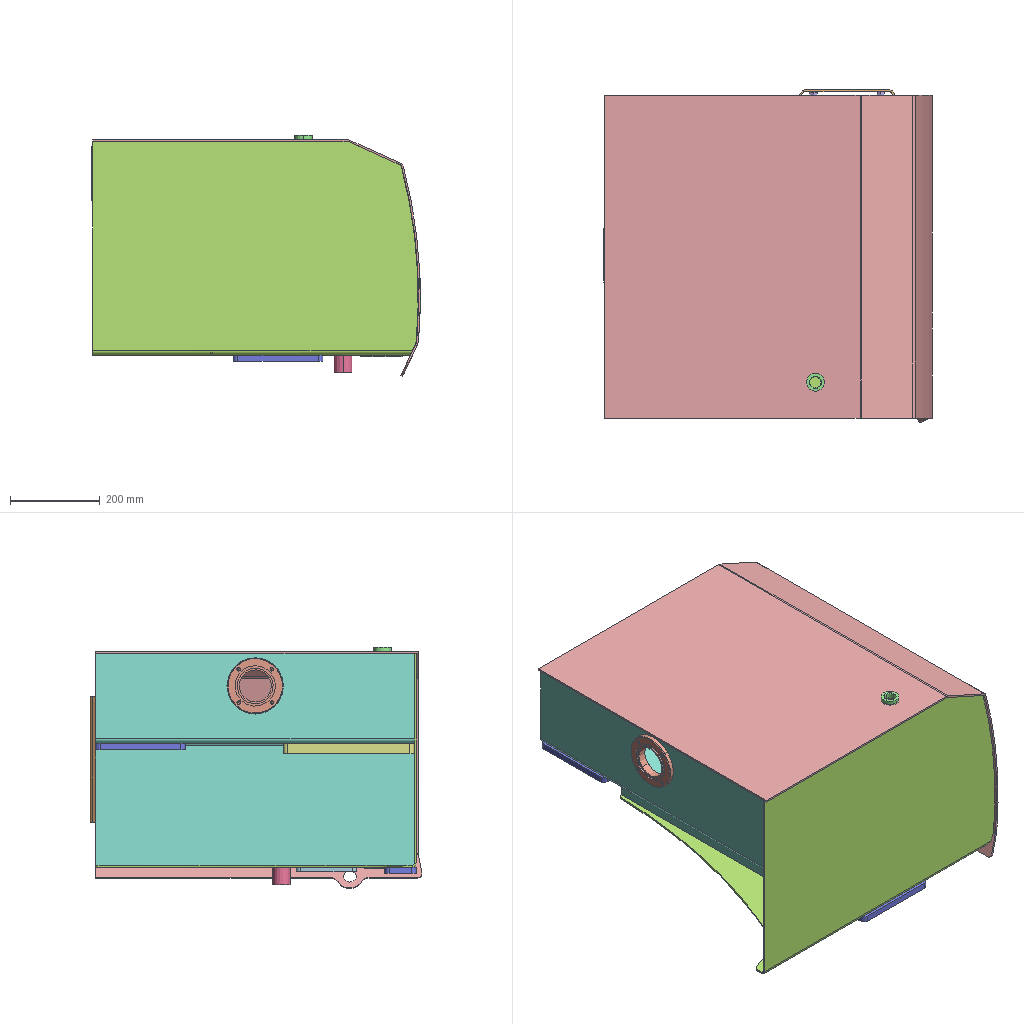Assembly | SolidWorks | 16 different items | 19 placed | box 733 x 740 x 538 mm
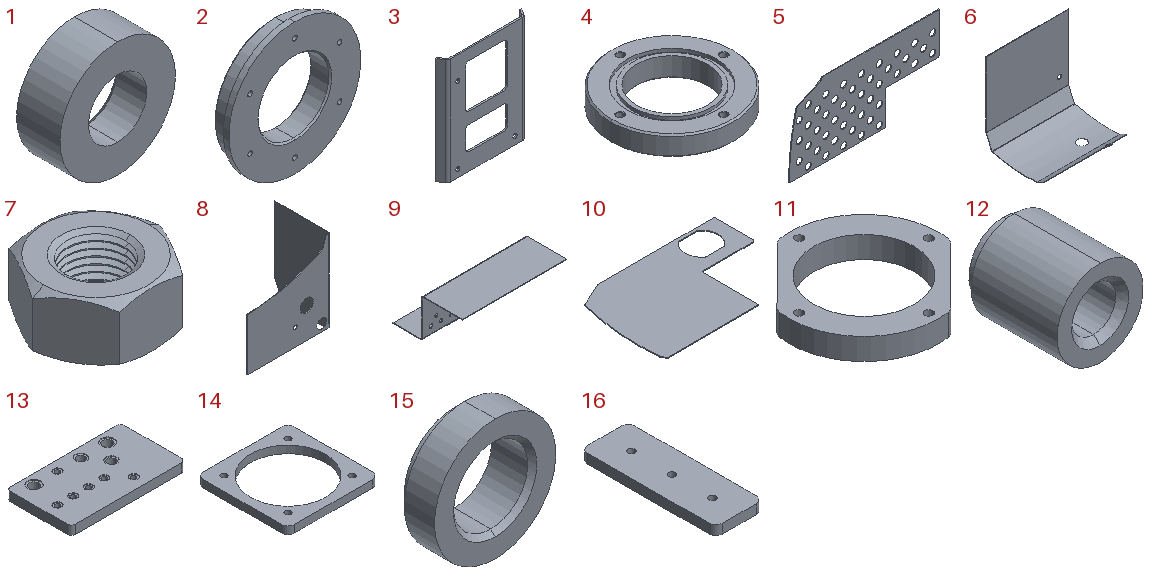Parts list (item | quantity | size | volume | features):
1 | x1 | 80 x 30 x 80 mm | 100918 mm3 | features HoleWzd 1, Revolution 1
2 | x1 | 93 x 14.5 x 93 mm | 57472 mm3 | features Chamfer 1, HoleWzd 1, Revolution 1
3 | x1 | 225 x 22.12 x 280 mm | 191805 mm3 | features FlatPattern 1, ICE 1, SMBaseFlange 1, SheetMetal 1
4 | x1 | 125 x 125 x 20 mm | 156275 mm3 | features Chamfer 2, ICE 2, FlatPattern 1, HoleWzd 1, SMBaseFlange 1, SheetMetal 1
5 | x1 | 714.557 x 4 x 360 mm | 695889 mm3 | features Extrusion 1
6 | x1 | 728.102 x 528.57 x 731.248 mm | 3316109 mm3 | features ICE 4, Fillet 1, FlatPattern 1, Fold 1, SMBaseFlange 1, SheetMetal 1, UnFold 1
7 | x3 | 18.475 x 16 x 8.4 mm | 1305 mm3 | features RevCut 2, Chamfer 1, Extrusion 1, LPattern 1
8 | x1 | 715 x 476 x 726.29 mm | 2754090 mm3 | features ICE 3, Fillet 2, FlatPattern 1, SMBaseFlange 1, SheetMetal 1
9 | x1 | 711 x 472 x 260 mm | 1991035 mm3 | features ICE 2, FlatPattern 1, SMBaseFlange 1, SheetMetal 1
10 | x1 | 714.283 x 472 x 4 mm | 956528 mm3 | features FlatPattern 1, SMBaseFlange 1, SheetMetal 1
11 | x1 | 158 x 158 x 23 mm | 204311 mm3 | features FlatPattern 1, HoleWzd 1, ICE 1, SMBaseFlange 1, SheetMetal 1
12 | x1 | 40 x 45 x 40 mm | 40970 mm3 | features Chamfer 1, Revolution 1
13 | x1 | 292 x 165 x 23 mm | 1047864 mm3 | features HoleWzd 4, ICE 3, FlatPattern 1, SMBaseFlange 1, SheetMetal 1
14 | x1 | 135 x 135 x 11 mm | 90588 mm3 | features FlatPattern 1, HoleWzd 1, SMBaseFlange 1, SheetMetal 1
15 | x1 | 40 x 13.5 x 40 mm | 9105 mm3 | features Chamfer 1, HoleWzd 1, Revolution 1
16 | x2 | 70 x 200 x 14 mm | 191366 mm3 | features FlatPattern 1, HoleWzd 1, SMBaseFlange 1, SheetMetal 1
Mates (type | each side: item.copy, entity, surface, feature):
Coincident | 6.1 face plane Base-Flange1 | 10.1 face plane Base-Flange1
DistanceDim | 6.1 face plane Base-Flange1 | 10.1 face plane Base-Flange1
DistanceDim | 10.1 face plane Base-Flange1 | 6.1 face plane Base-Flange1
Coincident | 6.1 face plane Base-Flange1 | 8.1 face plane Base-Flange1 | 2 times
DistanceDim | 8.1 face plane Base-Flange1 | 6.1 face plane Cut-Extrude2
Coincident | 6.1 face plane Base-Flange1 | 5.1 face plane Boss-Extrude1
DistanceDim | 6.1 face plane Base-Flange1 | 5.1 face plane Boss-Extrude1 | 2 times
Coincident | 10.1 face plane Base-Flange1 | 9.1 face plane Base-Flange1
Coincident | 6.1 face plane Base-Flange1 | 9.1 face plane Base-Flange1
Coincident | 8.1 face plane Base-Flange1 | 9.1 face plane Base-Flange1
DistanceDim | 10.1 face plane Base-Flange1 | 3.1 face plane Base-Flange1
DistanceDim | 9.1 face plane Base-Flange1 | 3.1 edge
DistanceDim | 8.1 face plane Base-Flange1 | 3.1 face plane Base-Flange1
Concentric | 3.1 face cylinder Cut-Extrude1 | 7.1 edge
Coincident | 3.1 face plane Base-Flange1 | 7.1 face plane BaseNut
Parallel | 7.1 face plane BaseNut | assembly plane
Coincident | 6.1 face plane Base-Flange1 | 15.1 face plane Revolve1
Concentric | 6.1 face cylinder Cut-Extrude3 | 15.1 face cylinder Revolve1
Parallel | 15.1 plane | assembly plane
Coincident | 8.1 face plane Base-Flange1 | 12.1 face plane Revolve1
Concentric | 8.1 face cylinder Cut-Extrude3 | 12.1 face cylinder Revolve1
Parallel | 12.1 plane | assembly plane
Coincident | 8.1 face plane Base-Flange1 | 14.1 face plane Base-Flange1
Concentric | 8.1 face cylinder Cut-Extrude3 | 14.1 face cylinder Base-Flange1
Parallel | 14.1 plane | assembly plane
Coincident | 9.1 face plane Base-Flange1 | 13.1 face plane Base-Flange1
Concentric | 13.1 face cylinder M26X1.5 Tapped Hole1 | 9.1 face cylinder Cut-Extrude2
Concentric | 9.1 face cylinder Cut-Extrude2 | 13.1 face cylinder M22x1.5 Tapped Hole1
Concentric | 10.1 face cylinder Base-Flange1 | 11.1 face cylinder Base-Flange1
Parallel | 10.1 face plane Base-Flange1 | 11.1 face plane Base-Flange1
DistanceDim | 11.1 face plane Base-Flange1 | 10.1 face plane Base-Flange1
Coincident | 8.1 face plane Base-Flange1 | 2.1 face plane Revolve1
Concentric | 8.1 face cylinder Cut-Extrude3 | 2.1 face cone Chamfer1
PlanarAngleDim | 2.1 plane | assembly plane
Concentric | 9.1 face cylinder Cut-Extrude1 | 4.1 face cylinder Base-Flange1
DistanceDim | 9.1 face plane Base-Flange1 | 4.1 face plane Base-Flange1
PlanarAngleDim | 4.1 plane | assembly plane
Coincident | 9.1 face plane Base-Flange1 | 16.1 face plane Base-Flange1 | 3 times
Coincident | 8.1 face plane Base-Flange1 | 16.2 face plane Base-Flange1 | 2 times
DistanceDim | 2.1 face cylinder Revolve1 | 16.2 face plane Base-Flange1
Tangent | 6.1 face surface:4006 Cut-Extrude4 | 1.1 face cylinder Revolve1
DistanceDim | 1.1 plane | assembly plane